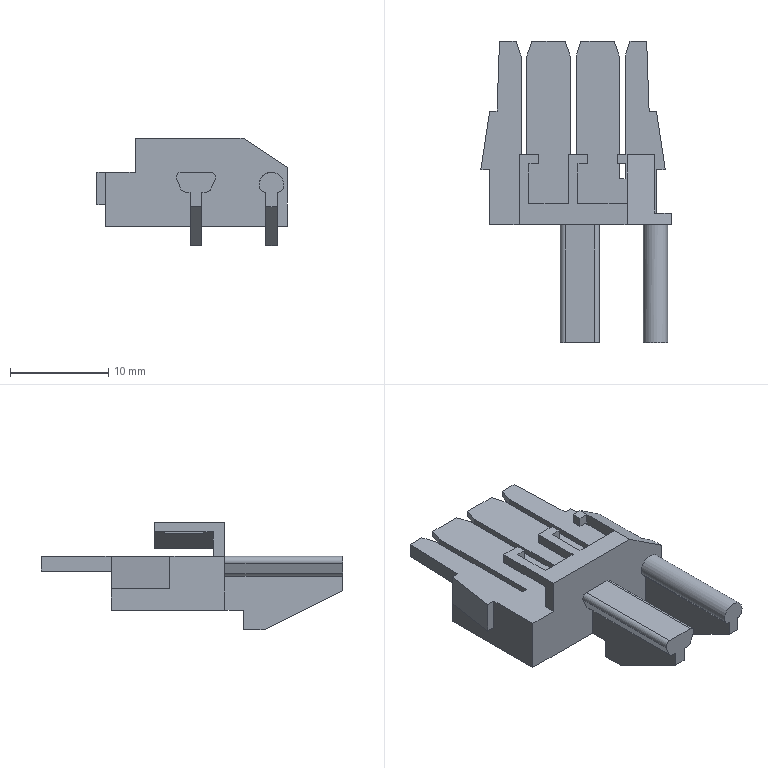Part | STEP file | LIANJIEQI1_17_1 | 1 solid | 148 faces | box 19.4 x 30.7 x 11 mm | volume 1115 mm3 | plane 141 | cylinder 7 | commonest cylinder face diameters 1 x6 2.5 x1